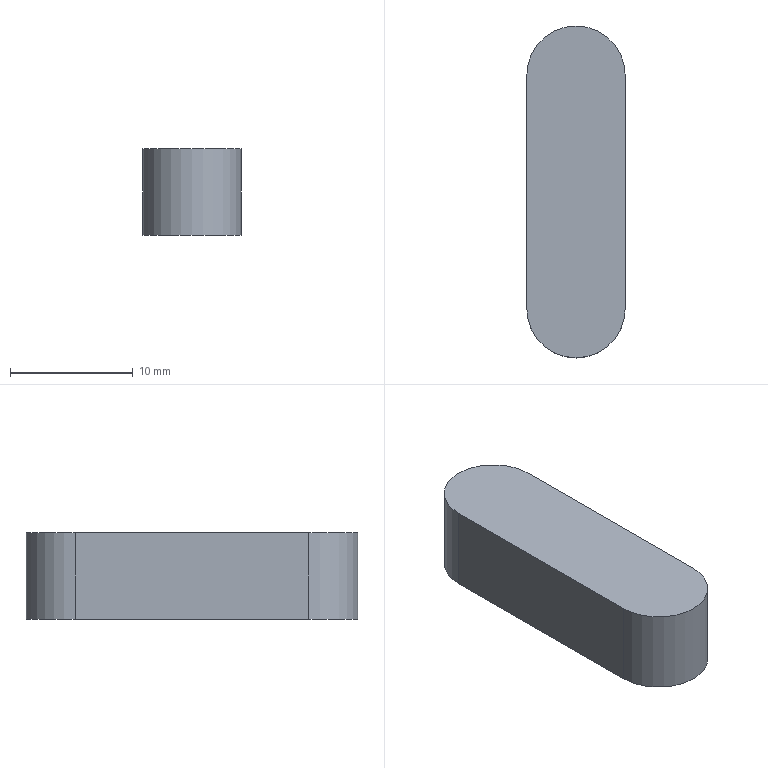Part | SolidWorks | features BaseBody 1 | 1 solid | 6 faces | box 8 x 27 x 7 mm | volume 1416 mm3 | plane 4 | cylinder 2 | commonest cylinder face diameters 8 x2
STEP:
#1=CARTESIAN_POINT('',(-4.,-19.,7.));
#2=VERTEX_POINT('',#1);
#3=CARTESIAN_POINT('',(4.,-19.,7.));
#4=VERTEX_POINT('',#3);
#5=CARTESIAN_POINT('',(0.,-19.,7.));
#6=DIRECTION('',(0.,0.,1.));
#7=DIRECTION('',(-1.,0.,0.));
#8=AXIS2_PLACEMENT_3D('',#5,#6,#7);
#9=CIRCLE('',#8,4.);
#10=EDGE_CURVE('',#2,#4,#9,.T.);
#11=ORIENTED_EDGE('',*,*,#10,.T.);
#12=CARTESIAN_POINT('',(4.,0.,7.));
#13=VERTEX_POINT('',#12);
#14=CARTESIAN_POINT('',(4.,0.,7.));
#15=DIRECTION('',(0.,1.,0.));
#16=VECTOR('',#15,1000.);
#17=LINE('',#14,#16);
#18=EDGE_CURVE('',#4,#13,#17,.T.);
#19=ORIENTED_EDGE('',*,*,#18,.T.);
#20=CARTESIAN_POINT('',(-4.,0.,7.));
#21=VERTEX_POINT('',#20);
#22=CARTESIAN_POINT('',(0.,0.,7.));
#23=DIRECTION('',(0.,0.,1.));
#24=DIRECTION('',(-1.,0.,0.));
#25=AXIS2_PLACEMENT_3D('',#22,#23,#24);
#26=CIRCLE('',#25,4.);
#27=EDGE_CURVE('',#13,#21,#26,.T.);
#28=ORIENTED_EDGE('',*,*,#27,.T.);
#29=CARTESIAN_POINT('',(-4.,0.,7.));
#30=DIRECTION('',(0.,-1.,0.));
#31=VECTOR('',#30,1000.);
#32=LINE('',#29,#31);
#33=EDGE_CURVE('',#21,#2,#32,.T.);
#34=ORIENTED_EDGE('',*,*,#33,.T.);
#35=EDGE_LOOP('',(#11,#19,#28,#34));
#36=FACE_OUTER_BOUND('',#35,.T.);
#37=CARTESIAN_POINT('',(0.,0.,7.));
#38=DIRECTION('',(0.,0.,1.));
#39=DIRECTION('',(1.,0.,0.));
#40=AXIS2_PLACEMENT_3D('',#37,#38,#39);
#41=PLANE('',#40);
#42=ADVANCED_FACE('',(#36),#41,.T.);
#43=CARTESIAN_POINT('',(4.,0.,0.));
#44=VERTEX_POINT('',#43);
#45=CARTESIAN_POINT('',(4.,0.,7.));
#46=DIRECTION('',(0.,0.,-1.));
#47=VECTOR('',#46,1000.);
#48=LINE('',#45,#47);
#49=EDGE_CURVE('',#13,#44,#48,.T.);
#50=ORIENTED_EDGE('',*,*,#49,.F.);
#51=ORIENTED_EDGE('',*,*,#18,.F.);
#52=CARTESIAN_POINT('',(4.,-19.,0.));
#53=VERTEX_POINT('',#52);
#54=CARTESIAN_POINT('',(4.,-19.,7.));
#55=DIRECTION('',(0.,0.,1.));
#56=VECTOR('',#55,1000.);
#57=LINE('',#54,#56);
#58=EDGE_CURVE('',#53,#4,#57,.T.);
#59=ORIENTED_EDGE('',*,*,#58,.F.);
#60=CARTESIAN_POINT('',(4.,0.,0.));
#61=DIRECTION('',(0.,-1.,0.));
#62=VECTOR('',#61,1000.);
#63=LINE('',#60,#62);
#64=EDGE_CURVE('',#44,#53,#63,.T.);
#65=ORIENTED_EDGE('',*,*,#64,.F.);
#66=EDGE_LOOP('',(#50,#51,#59,#65));
#67=FACE_OUTER_BOUND('',#66,.T.);
#68=CARTESIAN_POINT('',(4.,0.,7.));
#69=DIRECTION('',(-1.,0.,0.));
#70=DIRECTION('',(0.,-1.,0.));
#71=AXIS2_PLACEMENT_3D('',#68,#69,#70);
#72=PLANE('',#71);
#73=ADVANCED_FACE('',(#67),#72,.F.);
#74=ORIENTED_EDGE('',*,*,#10,.F.);
#75=CARTESIAN_POINT('',(-4.,-19.,0.));
#76=VERTEX_POINT('',#75);
#77=CARTESIAN_POINT('',(-4.,-19.,7.));
#78=DIRECTION('',(0.,0.,-1.));
#79=VECTOR('',#78,1000.);
#80=LINE('',#77,#79);
#81=EDGE_CURVE('',#2,#76,#80,.T.);
#82=ORIENTED_EDGE('',*,*,#81,.T.);
#83=CARTESIAN_POINT('',(0.,-19.,0.));
#84=DIRECTION('',(0.,0.,1.));
#85=DIRECTION('',(-1.,0.,0.));
#86=AXIS2_PLACEMENT_3D('',#83,#84,#85);
#87=CIRCLE('',#86,4.);
#88=EDGE_CURVE('',#76,#53,#87,.T.);
#89=ORIENTED_EDGE('',*,*,#88,.T.);
#90=ORIENTED_EDGE('',*,*,#58,.T.);
#91=EDGE_LOOP('',(#74,#82,#89,#90));
#92=FACE_OUTER_BOUND('',#91,.T.);
#93=CARTESIAN_POINT('',(0.,-19.,7.));
#94=DIRECTION('',(0.,0.,-1.));
#95=DIRECTION('',(-1.,0.,0.));
#96=AXIS2_PLACEMENT_3D('',#93,#94,#95);
#97=CYLINDRICAL_SURFACE('',#96,4.);
#98=ADVANCED_FACE('',(#92),#97,.T.);
#99=ORIENTED_EDGE('',*,*,#81,.F.);
#100=ORIENTED_EDGE('',*,*,#33,.F.);
#101=CARTESIAN_POINT('',(-4.,0.,0.));
#102=VERTEX_POINT('',#101);
#103=CARTESIAN_POINT('',(-4.,0.,7.));
#104=DIRECTION('',(0.,0.,1.));
#105=VECTOR('',#104,1000.);
#106=LINE('',#103,#105);
#107=EDGE_CURVE('',#102,#21,#106,.T.);
#108=ORIENTED_EDGE('',*,*,#107,.F.);
#109=CARTESIAN_POINT('',(-4.,0.,0.));
#110=DIRECTION('',(0.,1.,0.));
#111=VECTOR('',#110,1000.);
#112=LINE('',#109,#111);
#113=EDGE_CURVE('',#76,#102,#112,.T.);
#114=ORIENTED_EDGE('',*,*,#113,.F.);
#115=EDGE_LOOP('',(#99,#100,#108,#114));
#116=FACE_OUTER_BOUND('',#115,.T.);
#117=CARTESIAN_POINT('',(-4.,0.,7.));
#118=DIRECTION('',(1.,0.,0.));
#119=DIRECTION('',(0.,1.,0.));
#120=AXIS2_PLACEMENT_3D('',#117,#118,#119);
#121=PLANE('',#120);
#122=ADVANCED_FACE('',(#116),#121,.F.);
#123=ORIENTED_EDGE('',*,*,#27,.F.);
#124=ORIENTED_EDGE('',*,*,#49,.T.);
#125=CARTESIAN_POINT('',(0.,0.,0.));
#126=DIRECTION('',(0.,0.,1.));
#127=DIRECTION('',(-1.,0.,0.));
#128=AXIS2_PLACEMENT_3D('',#125,#126,#127);
#129=CIRCLE('',#128,4.);
#130=EDGE_CURVE('',#44,#102,#129,.T.);
#131=ORIENTED_EDGE('',*,*,#130,.T.);
#132=ORIENTED_EDGE('',*,*,#107,.T.);
#133=EDGE_LOOP('',(#123,#124,#131,#132));
#134=FACE_OUTER_BOUND('',#133,.T.);
#135=CARTESIAN_POINT('',(0.,0.,7.));
#136=DIRECTION('',(0.,0.,-1.));
#137=DIRECTION('',(-1.,0.,0.));
#138=AXIS2_PLACEMENT_3D('',#135,#136,#137);
#139=CYLINDRICAL_SURFACE('',#138,4.);
#140=ADVANCED_FACE('',(#134),#139,.T.);
#141=ORIENTED_EDGE('',*,*,#64,.T.);
#142=ORIENTED_EDGE('',*,*,#88,.F.);
#143=ORIENTED_EDGE('',*,*,#113,.T.);
#144=ORIENTED_EDGE('',*,*,#130,.F.);
#145=EDGE_LOOP('',(#141,#142,#143,#144));
#146=FACE_OUTER_BOUND('',#145,.T.);
#147=CARTESIAN_POINT('',(0.,0.,0.));
#148=DIRECTION('',(0.,0.,1.));
#149=DIRECTION('',(1.,0.,0.));
#150=AXIS2_PLACEMENT_3D('',#147,#148,#149);
#151=PLANE('',#150);
#152=ADVANCED_FACE('',(#146),#151,.F.);
#153=CLOSED_SHELL('',(#42,#73,#98,#122,#140,#152));
#154=MANIFOLD_SOLID_BREP('',#153);
#155=CARTESIAN_POINT('',(0.,0.,0.));
#156=DIRECTION('',(0.,0.,1.));
#157=DIRECTION('',(1.,0.,0.));
#158=AXIS2_PLACEMENT_3D('',#155,#156,#157);
#159=(LENGTH_UNIT()NAMED_UNIT(*)SI_UNIT(.MILLI.,.METRE.));
#160=UNCERTAINTY_MEASURE_WITH_UNIT(LENGTH_MEASURE(0.00001),#159,'','');
#161=(NAMED_UNIT(*)PLANE_ANGLE_UNIT()SI_UNIT($,.RADIAN.));
#162=(NAMED_UNIT(*)SI_UNIT($,.STERADIAN.)SOLID_ANGLE_UNIT());
#163=(GEOMETRIC_REPRESENTATION_CONTEXT(3)GLOBAL_UNCERTAINTY_ASSIGNED_CONTEXT((#160))GLOBAL_UNIT_ASSIGNED_CONTEXT((#159,#161,#162))REPRESENTATION_CONTEXT('',''));
#164=ADVANCED_BREP_SHAPE_REPRESENTATION('',(#154,#158),#163);